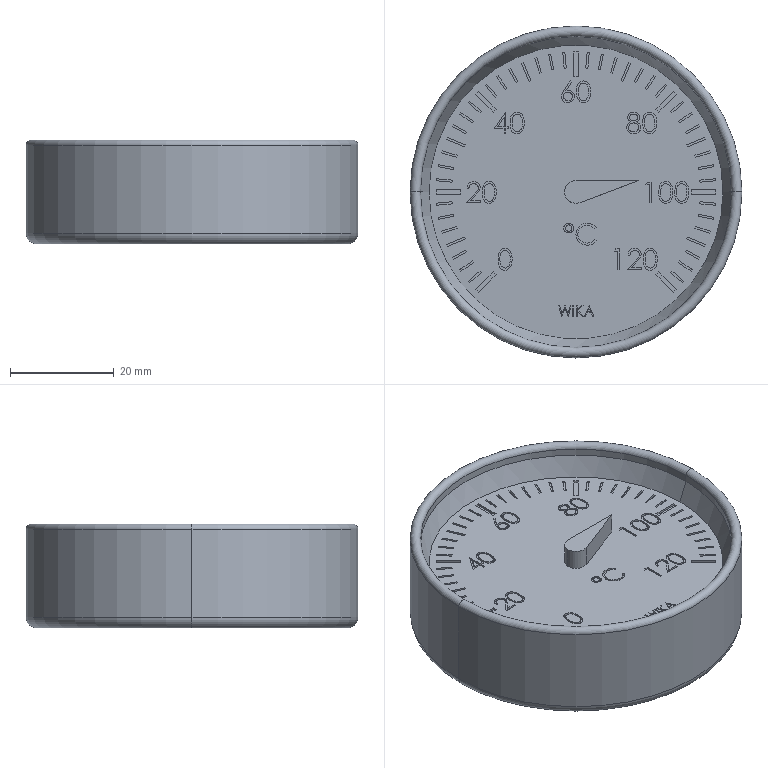Part | SolidWorks | features ICE 17, Fillet 3, CirPattern 1, Extrusion 1, MoveCopyBody 1, RevCut 1, Scale 1, Stock 1 | 1 solid | 519 faces | box 64 x 64 x 20 mm | volume 43695 mm3 | plane 368 | spline 127 | torus 12 | cylinder 6 | cone 6 | commonest cylinder face diameters 4.406 x2 60 x2 64 x2